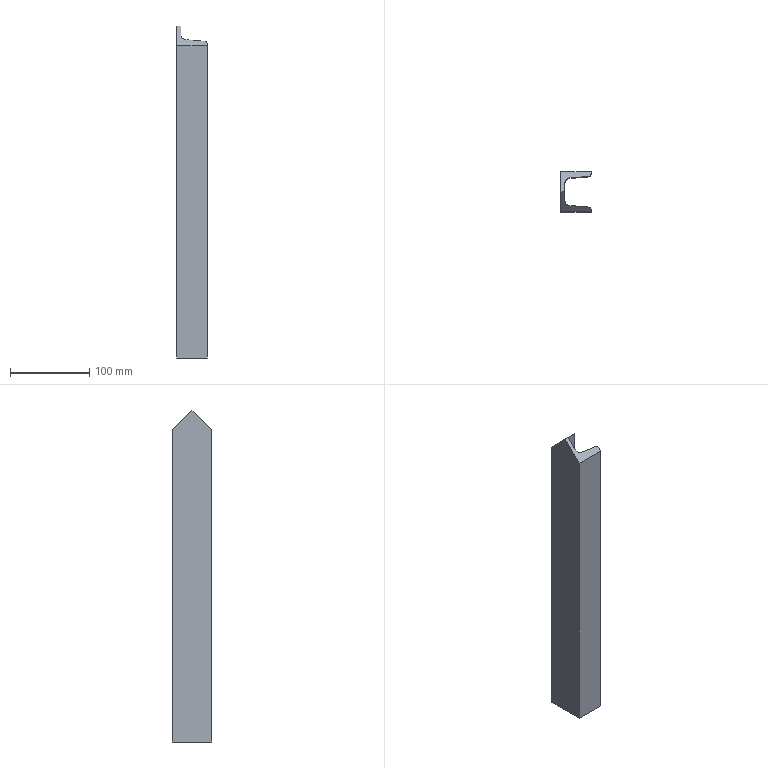Part | STEP file | DIN 1026-1 U 50 1785357045525 | 1 solid | 15 faces | box 38 x 50 x 417.981 mm | volume 284561 mm3 | plane 11 | cylinder 4 | commonest cylinder face diameters 7 x2 14 x2
STEP:
#1=CARTESIAN_POINT('',(0.,0.000000003,467.981));
#2=VERTEX_POINT('',#1);
#3=CARTESIAN_POINT('',(5.,0.000000003,467.981));
#4=VERTEX_POINT('',#3);
#5=CARTESIAN_POINT('',(9.5,0.000000003,467.981));
#6=DIRECTION('',(1.,0.,0.));
#7=VECTOR('',#6,10.);
#8=LINE('',#5,#7);
#9=EDGE_CURVE('',#2,#4,#8,.T.);
#10=ORIENTED_EDGE('',*,*,#9,.T.);
#11=CARTESIAN_POINT('',(5.,10.418,457.563));
#12=VERTEX_POINT('',#11);
#13=CARTESIAN_POINT('',(5.,233.99,233.99));
#14=DIRECTION('',(0.,-0.7071,0.7071));
#15=VECTOR('',#14,10.);
#16=LINE('',#13,#15);
#17=EDGE_CURVE('',#12,#4,#16,.T.);
#18=ORIENTED_EDGE('',*,*,#17,.F.);
#19=CARTESIAN_POINT('',(11.442,17.395,450.585));
#20=VERTEX_POINT('',#19);
#21=CARTESIAN_POINT('',(12.,10.418,457.563));
#22=DIRECTION('',(0.,0.7071,0.7071));
#23=DIRECTION('',(0.,0.7071,-0.7071));
#24=AXIS2_PLACEMENT_3D('',#21,#22,#23);
#25=ELLIPSE('',#24,9.899,7.);
#26=EDGE_CURVE('',#20,#12,#25,.T.);
#27=ORIENTED_EDGE('',*,*,#26,.F.);
#28=CARTESIAN_POINT('',(34.779,19.262,448.719));
#29=VERTEX_POINT('',#28);
#30=CARTESIAN_POINT('',(52.292,20.663,447.317));
#31=DIRECTION('',(-0.9937,-0.07949,0.07949));
#32=VECTOR('',#31,10.);
#33=LINE('',#30,#32);
#34=EDGE_CURVE('',#29,#20,#33,.T.);
#35=ORIENTED_EDGE('',*,*,#34,.F.);
#36=CARTESIAN_POINT('',(38.,22.751,445.23));
#37=VERTEX_POINT('',#36);
#38=CARTESIAN_POINT('',(34.5,22.751,445.23));
#39=DIRECTION('',(0.,-0.7071,-0.7071));
#40=DIRECTION('',(0.,0.7071,-0.7071));
#41=AXIS2_PLACEMENT_3D('',#38,#39,#40);
#42=ELLIPSE('',#41,4.95,3.5);
#43=EDGE_CURVE('',#37,#29,#42,.T.);
#44=ORIENTED_EDGE('',*,*,#43,.F.);
#45=CARTESIAN_POINT('',(38.,25.,442.981));
#46=VERTEX_POINT('',#45);
#47=CARTESIAN_POINT('',(38.,240.24,227.74));
#48=DIRECTION('',(0.,-0.7071,0.7071));
#49=VECTOR('',#48,10.);
#50=LINE('',#47,#49);
#51=EDGE_CURVE('',#46,#37,#50,.T.);
#52=ORIENTED_EDGE('',*,*,#51,.F.);
#53=CARTESIAN_POINT('',(0.,25.,442.981));
#54=VERTEX_POINT('',#53);
#55=CARTESIAN_POINT('',(0.,25.,442.981));
#56=DIRECTION('',(1.,0.,0.));
#57=VECTOR('',#56,10.);
#58=LINE('',#55,#57);
#59=EDGE_CURVE('',#54,#46,#58,.T.);
#60=ORIENTED_EDGE('',*,*,#59,.F.);
#61=CARTESIAN_POINT('',(0.,233.99,233.99));
#62=DIRECTION('',(0.,0.7071,-0.7071));
#63=VECTOR('',#62,10.);
#64=LINE('',#61,#63);
#65=EDGE_CURVE('',#2,#54,#64,.T.);
#66=ORIENTED_EDGE('',*,*,#65,.F.);
#67=EDGE_LOOP('',(#10,#18,#27,#35,#44,#52,#60,#66));
#68=FACE_OUTER_BOUND('',#67,.T.);
#69=CARTESIAN_POINT('',(0.,233.99,233.99));
#70=DIRECTION('',(0.,-0.7071,-0.7071));
#71=DIRECTION('',(-1.,0.,0.));
#72=AXIS2_PLACEMENT_3D('',#69,#70,#71);
#73=PLANE('',#72);
#74=ADVANCED_FACE('',(#68),#73,.F.);
#75=ORIENTED_EDGE('',*,*,#34,.T.);
#76=CARTESIAN_POINT('',(11.442,17.395,50.));
#77=VERTEX_POINT('',#76);
#78=CARTESIAN_POINT('',(11.442,17.395,0.));
#79=DIRECTION('',(0.,0.,1.));
#80=VECTOR('',#79,10.);
#81=LINE('',#78,#80);
#82=EDGE_CURVE('',#77,#20,#81,.T.);
#83=ORIENTED_EDGE('',*,*,#82,.F.);
#84=CARTESIAN_POINT('',(34.779,19.262,50.));
#85=VERTEX_POINT('',#84);
#86=CARTESIAN_POINT('',(26.174,18.574,50.));
#87=DIRECTION('',(-0.9968,-0.07975,0.));
#88=VECTOR('',#87,10.);
#89=LINE('',#86,#88);
#90=EDGE_CURVE('',#85,#77,#89,.T.);
#91=ORIENTED_EDGE('',*,*,#90,.F.);
#92=CARTESIAN_POINT('',(34.779,19.262,0.));
#93=DIRECTION('',(0.,0.,1.));
#94=VECTOR('',#93,10.);
#95=LINE('',#92,#94);
#96=EDGE_CURVE('',#85,#29,#95,.T.);
#97=ORIENTED_EDGE('',*,*,#96,.T.);
#98=EDGE_LOOP('',(#75,#83,#91,#97));
#99=FACE_OUTER_BOUND('',#98,.T.);
#100=CARTESIAN_POINT('',(34.779,19.262,0.));
#101=DIRECTION('',(0.07975,-0.9968,0.));
#102=DIRECTION('',(0.,0.,-1.));
#103=AXIS2_PLACEMENT_3D('',#100,#101,#102);
#104=PLANE('',#103);
#105=ADVANCED_FACE('',(#99),#104,.T.);
#106=ORIENTED_EDGE('',*,*,#26,.T.);
#107=CARTESIAN_POINT('',(5.,10.418,50.));
#108=VERTEX_POINT('',#107);
#109=CARTESIAN_POINT('',(5.,10.418,0.));
#110=DIRECTION('',(0.,0.,1.));
#111=VECTOR('',#110,10.);
#112=LINE('',#109,#111);
#113=EDGE_CURVE('',#108,#12,#112,.T.);
#114=ORIENTED_EDGE('',*,*,#113,.F.);
#115=CARTESIAN_POINT('',(12.,10.418,50.));
#116=DIRECTION('',(0.,0.,1.));
#117=DIRECTION('',(-0.07975,0.9968,0.));
#118=AXIS2_PLACEMENT_3D('',#115,#116,#117);
#119=CIRCLE('',#118,7.);
#120=EDGE_CURVE('',#77,#108,#119,.T.);
#121=ORIENTED_EDGE('',*,*,#120,.F.);
#122=ORIENTED_EDGE('',*,*,#82,.T.);
#123=EDGE_LOOP('',(#106,#114,#121,#122));
#124=FACE_OUTER_BOUND('',#123,.T.);
#125=CARTESIAN_POINT('',(12.,10.418,0.));
#126=DIRECTION('',(0.,0.,1.));
#127=DIRECTION('',(-0.07975,0.9968,0.));
#128=AXIS2_PLACEMENT_3D('',#125,#126,#127);
#129=CYLINDRICAL_SURFACE('',#128,7.);
#130=ADVANCED_FACE('',(#124),#129,.F.);
#131=ORIENTED_EDGE('',*,*,#17,.T.);
#132=CARTESIAN_POINT('',(5.,-10.418,457.563));
#133=VERTEX_POINT('',#132);
#134=CARTESIAN_POINT('',(5.,-233.99,233.99));
#135=DIRECTION('',(0.,-0.7071,-0.7071));
#136=VECTOR('',#135,10.);
#137=LINE('',#134,#136);
#138=EDGE_CURVE('',#4,#133,#137,.T.);
#139=ORIENTED_EDGE('',*,*,#138,.T.);
#140=CARTESIAN_POINT('',(5.,-10.418,50.));
#141=VERTEX_POINT('',#140);
#142=CARTESIAN_POINT('',(5.,-10.418,0.));
#143=DIRECTION('',(0.,0.,1.));
#144=VECTOR('',#143,10.);
#145=LINE('',#142,#144);
#146=EDGE_CURVE('',#141,#133,#145,.T.);
#147=ORIENTED_EDGE('',*,*,#146,.F.);
#148=CARTESIAN_POINT('',(5.,0.,50.));
#149=DIRECTION('',(0.,-1.,0.));
#150=VECTOR('',#149,10.);
#151=LINE('',#148,#150);
#152=EDGE_CURVE('',#108,#141,#151,.T.);
#153=ORIENTED_EDGE('',*,*,#152,.F.);
#154=ORIENTED_EDGE('',*,*,#113,.T.);
#155=EDGE_LOOP('',(#131,#139,#147,#153,#154));
#156=FACE_OUTER_BOUND('',#155,.T.);
#157=CARTESIAN_POINT('',(5.,0.,0.));
#158=DIRECTION('',(1.,0.,0.));
#159=DIRECTION('',(0.,0.,-1.));
#160=AXIS2_PLACEMENT_3D('',#157,#158,#159);
#161=PLANE('',#160);
#162=ADVANCED_FACE('',(#156),#161,.T.);
#163=CARTESIAN_POINT('',(11.442,-17.395,450.585));
#164=VERTEX_POINT('',#163);
#165=CARTESIAN_POINT('',(12.,-10.418,457.563));
#166=DIRECTION('',(0.,-0.7071,0.7071));
#167=DIRECTION('',(0.,-0.7071,-0.7071));
#168=AXIS2_PLACEMENT_3D('',#165,#166,#167);
#169=ELLIPSE('',#168,9.899,7.);
#170=EDGE_CURVE('',#133,#164,#169,.T.);
#171=ORIENTED_EDGE('',*,*,#170,.F.);
#172=ORIENTED_EDGE('',*,*,#138,.F.);
#173=ORIENTED_EDGE('',*,*,#9,.F.);
#174=CARTESIAN_POINT('',(0.,-25.,442.981));
#175=VERTEX_POINT('',#174);
#176=CARTESIAN_POINT('',(0.,-233.99,233.99));
#177=DIRECTION('',(0.,0.7071,0.7071));
#178=VECTOR('',#177,10.);
#179=LINE('',#176,#178);
#180=EDGE_CURVE('',#175,#2,#179,.T.);
#181=ORIENTED_EDGE('',*,*,#180,.F.);
#182=CARTESIAN_POINT('',(38.,-25.,442.981));
#183=VERTEX_POINT('',#182);
#184=CARTESIAN_POINT('',(19.,-25.,442.981));
#185=DIRECTION('',(-1.,0.,0.));
#186=VECTOR('',#185,10.);
#187=LINE('',#184,#186);
#188=EDGE_CURVE('',#183,#175,#187,.T.);
#189=ORIENTED_EDGE('',*,*,#188,.F.);
#190=CARTESIAN_POINT('',(38.,-22.751,445.23));
#191=VERTEX_POINT('',#190);
#192=CARTESIAN_POINT('',(38.,-239.678,228.303));
#193=DIRECTION('',(0.,-0.7071,-0.7071));
#194=VECTOR('',#193,10.);
#195=LINE('',#192,#194);
#196=EDGE_CURVE('',#191,#183,#195,.T.);
#197=ORIENTED_EDGE('',*,*,#196,.F.);
#198=CARTESIAN_POINT('',(34.779,-19.262,448.719));
#199=VERTEX_POINT('',#198);
#200=CARTESIAN_POINT('',(34.5,-22.751,445.23));
#201=DIRECTION('',(0.,0.7071,-0.7071));
#202=DIRECTION('',(0.,-0.7071,-0.7071));
#203=AXIS2_PLACEMENT_3D('',#200,#201,#202);
#204=ELLIPSE('',#203,4.95,3.5);
#205=EDGE_CURVE('',#199,#191,#204,.T.);
#206=ORIENTED_EDGE('',*,*,#205,.F.);
#207=CARTESIAN_POINT('',(40.697,-19.736,448.245));
#208=DIRECTION('',(0.9937,-0.07949,-0.07949));
#209=VECTOR('',#208,10.);
#210=LINE('',#207,#209);
#211=EDGE_CURVE('',#164,#199,#210,.T.);
#212=ORIENTED_EDGE('',*,*,#211,.F.);
#213=EDGE_LOOP('',(#171,#172,#173,#181,#189,#197,#206,#212));
#214=FACE_OUTER_BOUND('',#213,.T.);
#215=CARTESIAN_POINT('',(0.,-233.99,233.99));
#216=DIRECTION('',(0.,0.7071,-0.7071));
#217=DIRECTION('',(-1.,0.,0.));
#218=AXIS2_PLACEMENT_3D('',#215,#216,#217);
#219=PLANE('',#218);
#220=ADVANCED_FACE('',(#214),#219,.F.);
#221=ORIENTED_EDGE('',*,*,#188,.T.);
#222=CARTESIAN_POINT('',(0.,-25.,50.));
#223=VERTEX_POINT('',#222);
#224=CARTESIAN_POINT('',(0.,-25.,0.));
#225=DIRECTION('',(0.,0.,1.));
#226=VECTOR('',#225,10.);
#227=LINE('',#224,#226);
#228=EDGE_CURVE('',#223,#175,#227,.T.);
#229=ORIENTED_EDGE('',*,*,#228,.F.);
#230=CARTESIAN_POINT('',(38.,-25.,50.));
#231=VERTEX_POINT('',#230);
#232=CARTESIAN_POINT('',(28.5,-25.,50.));
#233=DIRECTION('',(-1.,0.,0.));
#234=VECTOR('',#233,10.);
#235=LINE('',#232,#234);
#236=EDGE_CURVE('',#231,#223,#235,.T.);
#237=ORIENTED_EDGE('',*,*,#236,.F.);
#238=CARTESIAN_POINT('',(38.,-25.,0.));
#239=DIRECTION('',(0.,0.,1.));
#240=VECTOR('',#239,10.);
#241=LINE('',#238,#240);
#242=EDGE_CURVE('',#231,#183,#241,.T.);
#243=ORIENTED_EDGE('',*,*,#242,.T.);
#244=EDGE_LOOP('',(#221,#229,#237,#243));
#245=FACE_OUTER_BOUND('',#244,.T.);
#246=CARTESIAN_POINT('',(38.,-25.,0.));
#247=DIRECTION('',(0.,-1.,0.));
#248=DIRECTION('',(0.,0.,-1.));
#249=AXIS2_PLACEMENT_3D('',#246,#247,#248);
#250=PLANE('',#249);
#251=ADVANCED_FACE('',(#245),#250,.T.);
#252=ORIENTED_EDGE('',*,*,#65,.T.);
#253=CARTESIAN_POINT('',(0.,25.,50.));
#254=VERTEX_POINT('',#253);
#255=CARTESIAN_POINT('',(0.,25.,0.));
#256=DIRECTION('',(0.,0.,1.));
#257=VECTOR('',#256,10.);
#258=LINE('',#255,#257);
#259=EDGE_CURVE('',#254,#54,#258,.T.);
#260=ORIENTED_EDGE('',*,*,#259,.F.);
#261=CARTESIAN_POINT('',(0.,0.,50.));
#262=DIRECTION('',(0.,1.,0.));
#263=VECTOR('',#262,10.);
#264=LINE('',#261,#263);
#265=EDGE_CURVE('',#223,#254,#264,.T.);
#266=ORIENTED_EDGE('',*,*,#265,.F.);
#267=ORIENTED_EDGE('',*,*,#228,.T.);
#268=ORIENTED_EDGE('',*,*,#180,.T.);
#269=EDGE_LOOP('',(#252,#260,#266,#267,#268));
#270=FACE_OUTER_BOUND('',#269,.T.);
#271=CARTESIAN_POINT('',(0.,0.,0.));
#272=DIRECTION('',(-1.,0.,0.));
#273=DIRECTION('',(0.,0.,1.));
#274=AXIS2_PLACEMENT_3D('',#271,#272,#273);
#275=PLANE('',#274);
#276=ADVANCED_FACE('',(#270),#275,.T.);
#277=ORIENTED_EDGE('',*,*,#170,.T.);
#278=CARTESIAN_POINT('',(11.442,-17.395,50.));
#279=VERTEX_POINT('',#278);
#280=CARTESIAN_POINT('',(11.442,-17.395,0.));
#281=DIRECTION('',(0.,0.,1.));
#282=VECTOR('',#281,10.);
#283=LINE('',#280,#282);
#284=EDGE_CURVE('',#279,#164,#283,.T.);
#285=ORIENTED_EDGE('',*,*,#284,.F.);
#286=CARTESIAN_POINT('',(12.,-10.418,50.));
#287=DIRECTION('',(0.,0.,1.));
#288=DIRECTION('',(-1.,0.,0.));
#289=AXIS2_PLACEMENT_3D('',#286,#287,#288);
#290=CIRCLE('',#289,7.);
#291=EDGE_CURVE('',#141,#279,#290,.T.);
#292=ORIENTED_EDGE('',*,*,#291,.F.);
#293=ORIENTED_EDGE('',*,*,#146,.T.);
#294=EDGE_LOOP('',(#277,#285,#292,#293));
#295=FACE_OUTER_BOUND('',#294,.T.);
#296=CARTESIAN_POINT('',(12.,-10.418,0.));
#297=DIRECTION('',(0.,0.,1.));
#298=DIRECTION('',(-1.,0.,0.));
#299=AXIS2_PLACEMENT_3D('',#296,#297,#298);
#300=CYLINDRICAL_SURFACE('',#299,7.);
#301=ADVANCED_FACE('',(#295),#300,.F.);
#302=ORIENTED_EDGE('',*,*,#211,.T.);
#303=CARTESIAN_POINT('',(34.779,-19.262,50.));
#304=VERTEX_POINT('',#303);
#305=CARTESIAN_POINT('',(34.779,-19.262,0.));
#306=DIRECTION('',(0.,0.,1.));
#307=VECTOR('',#306,10.);
#308=LINE('',#305,#307);
#309=EDGE_CURVE('',#304,#199,#308,.T.);
#310=ORIENTED_EDGE('',*,*,#309,.F.);
#311=CARTESIAN_POINT('',(14.505,-17.64,50.));
#312=DIRECTION('',(0.9968,-0.07975,0.));
#313=VECTOR('',#312,10.);
#314=LINE('',#311,#313);
#315=EDGE_CURVE('',#279,#304,#314,.T.);
#316=ORIENTED_EDGE('',*,*,#315,.F.);
#317=ORIENTED_EDGE('',*,*,#284,.T.);
#318=EDGE_LOOP('',(#302,#310,#316,#317));
#319=FACE_OUTER_BOUND('',#318,.T.);
#320=CARTESIAN_POINT('',(11.442,-17.395,0.));
#321=DIRECTION('',(0.07975,0.9968,0.));
#322=DIRECTION('',(0.,0.,1.));
#323=AXIS2_PLACEMENT_3D('',#320,#321,#322);
#324=PLANE('',#323);
#325=ADVANCED_FACE('',(#319),#324,.T.);
#326=ORIENTED_EDGE('',*,*,#205,.T.);
#327=CARTESIAN_POINT('',(38.,-22.751,50.));
#328=VERTEX_POINT('',#327);
#329=CARTESIAN_POINT('',(38.,-22.751,0.));
#330=DIRECTION('',(0.,0.,1.));
#331=VECTOR('',#330,10.);
#332=LINE('',#329,#331);
#333=EDGE_CURVE('',#328,#191,#332,.T.);
#334=ORIENTED_EDGE('',*,*,#333,.F.);
#335=CARTESIAN_POINT('',(34.5,-22.751,50.));
#336=DIRECTION('',(0.,0.,-1.));
#337=DIRECTION('',(-1.,0.,0.));
#338=AXIS2_PLACEMENT_3D('',#335,#336,#337);
#339=CIRCLE('',#338,3.5);
#340=EDGE_CURVE('',#304,#328,#339,.T.);
#341=ORIENTED_EDGE('',*,*,#340,.F.);
#342=ORIENTED_EDGE('',*,*,#309,.T.);
#343=EDGE_LOOP('',(#326,#334,#341,#342));
#344=FACE_OUTER_BOUND('',#343,.T.);
#345=CARTESIAN_POINT('',(34.5,-22.751,0.));
#346=DIRECTION('',(0.,0.,1.));
#347=DIRECTION('',(-1.,0.,0.));
#348=AXIS2_PLACEMENT_3D('',#345,#346,#347);
#349=CYLINDRICAL_SURFACE('',#348,3.5);
#350=ADVANCED_FACE('',(#344),#349,.T.);
#351=ORIENTED_EDGE('',*,*,#196,.T.);
#352=ORIENTED_EDGE('',*,*,#242,.F.);
#353=CARTESIAN_POINT('',(38.,-11.376,50.));
#354=DIRECTION('',(0.,-1.,0.));
#355=VECTOR('',#354,10.);
#356=LINE('',#353,#355);
#357=EDGE_CURVE('',#328,#231,#356,.T.);
#358=ORIENTED_EDGE('',*,*,#357,.F.);
#359=ORIENTED_EDGE('',*,*,#333,.T.);
#360=EDGE_LOOP('',(#351,#352,#358,#359));
#361=FACE_OUTER_BOUND('',#360,.T.);
#362=CARTESIAN_POINT('',(38.,-22.751,0.));
#363=DIRECTION('',(1.,0.,0.));
#364=DIRECTION('',(0.,0.,-1.));
#365=AXIS2_PLACEMENT_3D('',#362,#363,#364);
#366=PLANE('',#365);
#367=ADVANCED_FACE('',(#361),#366,.T.);
#368=ORIENTED_EDGE('',*,*,#59,.T.);
#369=CARTESIAN_POINT('',(38.,25.,50.));
#370=VERTEX_POINT('',#369);
#371=CARTESIAN_POINT('',(38.,25.,0.));
#372=DIRECTION('',(0.,0.,1.));
#373=VECTOR('',#372,10.);
#374=LINE('',#371,#373);
#375=EDGE_CURVE('',#370,#46,#374,.T.);
#376=ORIENTED_EDGE('',*,*,#375,.F.);
#377=CARTESIAN_POINT('',(9.5,25.,50.));
#378=DIRECTION('',(1.,0.,0.));
#379=VECTOR('',#378,10.);
#380=LINE('',#377,#379);
#381=EDGE_CURVE('',#254,#370,#380,.T.);
#382=ORIENTED_EDGE('',*,*,#381,.F.);
#383=ORIENTED_EDGE('',*,*,#259,.T.);
#384=EDGE_LOOP('',(#368,#376,#382,#383));
#385=FACE_OUTER_BOUND('',#384,.T.);
#386=CARTESIAN_POINT('',(0.,25.,0.));
#387=DIRECTION('',(0.,1.,0.));
#388=DIRECTION('',(0.,0.,1.));
#389=AXIS2_PLACEMENT_3D('',#386,#387,#388);
#390=PLANE('',#389);
#391=ADVANCED_FACE('',(#385),#390,.T.);
#392=ORIENTED_EDGE('',*,*,#51,.T.);
#393=CARTESIAN_POINT('',(38.,22.751,50.));
#394=VERTEX_POINT('',#393);
#395=CARTESIAN_POINT('',(38.,22.751,0.));
#396=DIRECTION('',(0.,0.,1.));
#397=VECTOR('',#396,10.);
#398=LINE('',#395,#397);
#399=EDGE_CURVE('',#394,#37,#398,.T.);
#400=ORIENTED_EDGE('',*,*,#399,.F.);
#401=CARTESIAN_POINT('',(38.,12.5,50.));
#402=DIRECTION('',(0.,-1.,0.));
#403=VECTOR('',#402,10.);
#404=LINE('',#401,#403);
#405=EDGE_CURVE('',#370,#394,#404,.T.);
#406=ORIENTED_EDGE('',*,*,#405,.F.);
#407=ORIENTED_EDGE('',*,*,#375,.T.);
#408=EDGE_LOOP('',(#392,#400,#406,#407));
#409=FACE_OUTER_BOUND('',#408,.T.);
#410=CARTESIAN_POINT('',(38.,25.,0.));
#411=DIRECTION('',(1.,0.,0.));
#412=DIRECTION('',(0.,0.,-1.));
#413=AXIS2_PLACEMENT_3D('',#410,#411,#412);
#414=PLANE('',#413);
#415=ADVANCED_FACE('',(#409),#414,.T.);
#416=ORIENTED_EDGE('',*,*,#43,.T.);
#417=ORIENTED_EDGE('',*,*,#96,.F.);
#418=CARTESIAN_POINT('',(34.5,22.751,50.));
#419=DIRECTION('',(0.,0.,-1.));
#420=DIRECTION('',(-0.07975,0.9968,0.));
#421=AXIS2_PLACEMENT_3D('',#418,#419,#420);
#422=CIRCLE('',#421,3.5);
#423=EDGE_CURVE('',#394,#85,#422,.T.);
#424=ORIENTED_EDGE('',*,*,#423,.F.);
#425=ORIENTED_EDGE('',*,*,#399,.T.);
#426=EDGE_LOOP('',(#416,#417,#424,#425));
#427=FACE_OUTER_BOUND('',#426,.T.);
#428=CARTESIAN_POINT('',(34.5,22.751,0.));
#429=DIRECTION('',(0.,0.,1.));
#430=DIRECTION('',(-0.07975,0.9968,0.));
#431=AXIS2_PLACEMENT_3D('',#428,#429,#430);
#432=CYLINDRICAL_SURFACE('',#431,3.5);
#433=ADVANCED_FACE('',(#427),#432,.T.);
#434=ORIENTED_EDGE('',*,*,#381,.T.);
#435=ORIENTED_EDGE('',*,*,#405,.T.);
#436=ORIENTED_EDGE('',*,*,#423,.T.);
#437=ORIENTED_EDGE('',*,*,#90,.T.);
#438=ORIENTED_EDGE('',*,*,#120,.T.);
#439=ORIENTED_EDGE('',*,*,#152,.T.);
#440=ORIENTED_EDGE('',*,*,#291,.T.);
#441=ORIENTED_EDGE('',*,*,#315,.T.);
#442=ORIENTED_EDGE('',*,*,#340,.T.);
#443=ORIENTED_EDGE('',*,*,#357,.T.);
#444=ORIENTED_EDGE('',*,*,#236,.T.);
#445=ORIENTED_EDGE('',*,*,#265,.T.);
#446=EDGE_LOOP('',(#434,#435,#436,#437,#438,#439,#440,#441,#442,#443,#444,#445));
#447=FACE_OUTER_BOUND('',#446,.T.);
#448=CARTESIAN_POINT('',(19.,0.,50.));
#449=DIRECTION('',(0.,0.,1.));
#450=DIRECTION('',(1.,0.,0.));
#451=AXIS2_PLACEMENT_3D('',#448,#449,#450);
#452=PLANE('',#451);
#453=ADVANCED_FACE('',(#447),#452,.F.);
#454=CLOSED_SHELL('',(#74,#105,#130,#162,#220,#251,#276,#301,#325,#350,#367,#391,#415,#433,#453));
#455=MANIFOLD_SOLID_BREP('',#454);
#456=(LENGTH_UNIT()NAMED_UNIT(*)SI_UNIT(.MILLI.,.METRE.));
#457=UNCERTAINTY_MEASURE_WITH_UNIT(LENGTH_MEASURE(0.01),#456,'','');
#458=(NAMED_UNIT(*)PLANE_ANGLE_UNIT()SI_UNIT($,.RADIAN.));
#459=(NAMED_UNIT(*)SI_UNIT($,.STERADIAN.)SOLID_ANGLE_UNIT());
#460=(GEOMETRIC_REPRESENTATION_CONTEXT(3)GLOBAL_UNCERTAINTY_ASSIGNED_CONTEXT((#457))GLOBAL_UNIT_ASSIGNED_CONTEXT((#456,#458,#459))REPRESENTATION_CONTEXT('',''));
#461=ADVANCED_BREP_SHAPE_REPRESENTATION('',(#455),#460);